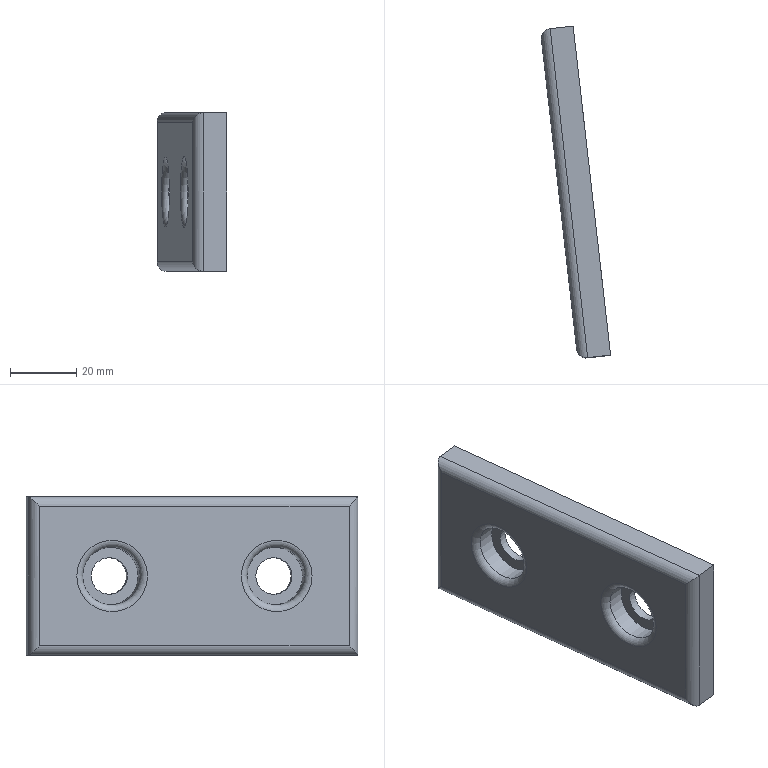Part | NX | features solid 2 | 1 solid | 18 faces | box 20.936 x 100.169 x 48 mm | volume 43256 mm3 | plane 8 | cylinder 8 | torus 2 | commonest cylinder face diameters 6 x4 11 x2 17.5 x2
STEP:
#1=CARTESIAN_POINT('',(3461.731,359.26,-59.));
#2=VERTEX_POINT('',#1);
#3=CARTESIAN_POINT('',(3462.354,353.796,-59.));
#4=DIRECTION('',(-0.9936,-0.1132,0.));
#5=DIRECTION('',(-0.1132,0.9936,0.));
#6=AXIS2_PLACEMENT_3D('',#3,#4,#5);
#7=CIRCLE('',#6,5.5);
#8=EDGE_CURVE('',#2,#2,#7,.T.);
#9=ORIENTED_EDGE('',*,*,#8,.T.);
#10=EDGE_LOOP('',(#9));
#11=FACE_BOUND('',#10,.T.);
#12=CARTESIAN_POINT('',(3467.392,309.582,-59.));
#13=VERTEX_POINT('',#12);
#14=CARTESIAN_POINT('',(3468.014,304.117,-59.));
#15=DIRECTION('',(-0.9936,-0.1132,0.));
#16=DIRECTION('',(-0.1132,0.9936,0.));
#17=AXIS2_PLACEMENT_3D('',#14,#15,#16);
#18=CIRCLE('',#17,5.5);
#19=EDGE_CURVE('',#13,#13,#18,.T.);
#20=ORIENTED_EDGE('',*,*,#19,.T.);
#21=EDGE_LOOP('',(#20));
#22=FACE_BOUND('',#21,.T.);
#23=CARTESIAN_POINT('',(3470.844,279.278,-35.));
#24=VERTEX_POINT('',#23);
#25=CARTESIAN_POINT('',(3470.844,279.278,-83.));
#26=VERTEX_POINT('',#25);
#27=CARTESIAN_POINT('',(3470.844,279.278,-59.));
#28=DIRECTION('',(0.,0.,-1.));
#29=VECTOR('',#28,1000.);
#30=LINE('',#27,#29);
#31=EDGE_CURVE('',#24,#26,#30,.T.);
#32=ORIENTED_EDGE('',*,*,#31,.T.);
#33=CARTESIAN_POINT('',(3459.524,378.635,-83.));
#34=VERTEX_POINT('',#33);
#35=CARTESIAN_POINT('',(3456.694,403.474,-83.));
#36=DIRECTION('',(0.1132,-0.9936,0.));
#37=VECTOR('',#36,1000.);
#38=LINE('',#35,#37);
#39=EDGE_CURVE('',#34,#26,#38,.T.);
#40=ORIENTED_EDGE('',*,*,#39,.F.);
#41=CARTESIAN_POINT('',(3459.524,378.635,-35.));
#42=VERTEX_POINT('',#41);
#43=CARTESIAN_POINT('',(3459.524,378.635,-59.));
#44=DIRECTION('',(0.,0.,1.));
#45=VECTOR('',#44,1000.);
#46=LINE('',#43,#45);
#47=EDGE_CURVE('',#34,#42,#46,.T.);
#48=ORIENTED_EDGE('',*,*,#47,.T.);
#49=CARTESIAN_POINT('',(3456.694,403.474,-35.));
#50=DIRECTION('',(0.1132,-0.9936,0.));
#51=VECTOR('',#50,1000.);
#52=LINE('',#49,#51);
#53=EDGE_CURVE('',#42,#24,#52,.T.);
#54=ORIENTED_EDGE('',*,*,#53,.T.);
#55=EDGE_LOOP('',(#32,#40,#48,#54));
#56=FACE_BOUND('',#55,.T.);
#57=CARTESIAN_POINT('',(3456.694,403.474,-59.));
#58=DIRECTION('',(0.9936,0.1132,0.));
#59=DIRECTION('',(0.1132,-0.9936,0.));
#60=AXIS2_PLACEMENT_3D('',#57,#58,#59);
#61=PLANE('',#60);
#62=ADVANCED_FACE('',(#11,#22,#56),#61,.T.);
#63=ORIENTED_EDGE('',*,*,#39,.T.);
#64=CARTESIAN_POINT('',(3463.889,278.485,-83.));
#65=VERTEX_POINT('',#64);
#66=CARTESIAN_POINT('',(3465.876,278.712,-83.));
#67=DIRECTION('',(-0.9936,-0.1132,0.));
#68=VECTOR('',#67,1000.);
#69=LINE('',#66,#68);
#70=EDGE_CURVE('',#26,#65,#69,.T.);
#71=ORIENTED_EDGE('',*,*,#70,.T.);
#72=CARTESIAN_POINT('',(3452.569,377.842,-83.));
#73=VERTEX_POINT('',#72);
#74=CARTESIAN_POINT('',(3449.739,402.682,-83.));
#75=DIRECTION('',(-0.1132,0.9936,0.));
#76=VECTOR('',#75,1000.);
#77=LINE('',#74,#76);
#78=EDGE_CURVE('',#65,#73,#77,.T.);
#79=ORIENTED_EDGE('',*,*,#78,.T.);
#80=CARTESIAN_POINT('',(3454.556,378.069,-83.));
#81=DIRECTION('',(0.9936,0.1132,0.));
#82=VECTOR('',#81,1000.);
#83=LINE('',#80,#82);
#84=EDGE_CURVE('',#73,#34,#83,.T.);
#85=ORIENTED_EDGE('',*,*,#84,.T.);
#86=EDGE_LOOP('',(#63,#71,#79,#85));
#87=FACE_BOUND('',#86,.T.);
#88=CARTESIAN_POINT('',(3451.726,402.908,-83.));
#89=DIRECTION('',(0.,0.,-1.));
#90=DIRECTION('',(-0.1132,0.9936,0.));
#91=AXIS2_PLACEMENT_3D('',#88,#89,#90);
#92=PLANE('',#91);
#93=ADVANCED_FACE('',(#87),#92,.T.);
#94=ORIENTED_EDGE('',*,*,#31,.F.);
#95=CARTESIAN_POINT('',(3463.889,278.485,-35.));
#96=VERTEX_POINT('',#95);
#97=CARTESIAN_POINT('',(3465.876,278.712,-35.));
#98=DIRECTION('',(0.9936,0.1132,0.));
#99=VECTOR('',#98,1000.);
#100=LINE('',#97,#99);
#101=EDGE_CURVE('',#96,#24,#100,.T.);
#102=ORIENTED_EDGE('',*,*,#101,.F.);
#103=CARTESIAN_POINT('',(3463.889,278.485,-59.));
#104=DIRECTION('',(0.,0.,-1.));
#105=VECTOR('',#104,1000.);
#106=LINE('',#103,#105);
#107=EDGE_CURVE('',#96,#65,#106,.T.);
#108=ORIENTED_EDGE('',*,*,#107,.T.);
#109=ORIENTED_EDGE('',*,*,#70,.F.);
#110=EDGE_LOOP('',(#94,#102,#108,#109));
#111=FACE_BOUND('',#110,.T.);
#112=CARTESIAN_POINT('',(3465.876,278.712,-59.));
#113=DIRECTION('',(0.1132,-0.9936,0.));
#114=DIRECTION('',(0.,0.,-1.));
#115=AXIS2_PLACEMENT_3D('',#112,#113,#114);
#116=PLANE('',#115);
#117=ADVANCED_FACE('',(#111),#116,.T.);
#118=CARTESIAN_POINT('',(3456.862,313.666,-59.));
#119=VERTEX_POINT('',#118);
#120=CARTESIAN_POINT('',(3458.078,302.985,-59.));
#121=DIRECTION('',(0.9936,0.1132,0.));
#122=DIRECTION('',(-0.1132,0.9936,0.));
#123=AXIS2_PLACEMENT_3D('',#120,#121,#122);
#124=CIRCLE('',#123,10.75);
#125=EDGE_CURVE('',#119,#119,#124,.T.);
#126=ORIENTED_EDGE('',*,*,#125,.T.);
#127=EDGE_LOOP('',(#126));
#128=FACE_BOUND('',#127,.T.);
#129=CARTESIAN_POINT('',(3451.201,363.344,-59.));
#130=VERTEX_POINT('',#129);
#131=CARTESIAN_POINT('',(3452.418,352.664,-59.));
#132=DIRECTION('',(0.9936,0.1132,0.));
#133=DIRECTION('',(-0.1132,0.9936,0.));
#134=AXIS2_PLACEMENT_3D('',#131,#132,#133);
#135=CIRCLE('',#134,10.75);
#136=EDGE_CURVE('',#130,#130,#135,.T.);
#137=ORIENTED_EDGE('',*,*,#136,.T.);
#138=EDGE_LOOP('',(#137));
#139=FACE_BOUND('',#138,.T.);
#140=CARTESIAN_POINT('',(3460.569,281.126,-38.));
#141=VERTEX_POINT('',#140);
#142=CARTESIAN_POINT('',(3449.928,374.522,-38.));
#143=VERTEX_POINT('',#142);
#144=CARTESIAN_POINT('',(3446.758,402.342,-38.));
#145=DIRECTION('',(-0.1132,0.9936,0.));
#146=VECTOR('',#145,1000.);
#147=LINE('',#144,#146);
#148=EDGE_CURVE('',#141,#143,#147,.T.);
#149=ORIENTED_EDGE('',*,*,#148,.T.);
#150=CARTESIAN_POINT('',(3449.928,374.522,-80.));
#151=VERTEX_POINT('',#150);
#152=CARTESIAN_POINT('',(3449.928,374.522,-59.));
#153=DIRECTION('',(0.,0.,-1.));
#154=VECTOR('',#153,1000.);
#155=LINE('',#152,#154);
#156=EDGE_CURVE('',#143,#151,#155,.T.);
#157=ORIENTED_EDGE('',*,*,#156,.T.);
#158=CARTESIAN_POINT('',(3460.569,281.126,-80.));
#159=VERTEX_POINT('',#158);
#160=CARTESIAN_POINT('',(3446.758,402.342,-80.));
#161=DIRECTION('',(0.1132,-0.9936,0.));
#162=VECTOR('',#161,1000.);
#163=LINE('',#160,#162);
#164=EDGE_CURVE('',#151,#159,#163,.T.);
#165=ORIENTED_EDGE('',*,*,#164,.T.);
#166=CARTESIAN_POINT('',(3460.569,281.126,-59.));
#167=DIRECTION('',(0.,0.,1.));
#168=VECTOR('',#167,1000.);
#169=LINE('',#166,#168);
#170=EDGE_CURVE('',#159,#141,#169,.T.);
#171=ORIENTED_EDGE('',*,*,#170,.T.);
#172=EDGE_LOOP('',(#149,#157,#165,#171));
#173=FACE_BOUND('',#172,.T.);
#174=CARTESIAN_POINT('',(3446.758,402.342,-59.));
#175=DIRECTION('',(-0.9936,-0.1132,0.));
#176=DIRECTION('',(-0.1132,0.9936,0.));
#177=AXIS2_PLACEMENT_3D('',#174,#175,#176);
#178=PLANE('',#177);
#179=ADVANCED_FACE('',(#128,#139,#173),#178,.T.);
#180=ORIENTED_EDGE('',*,*,#53,.F.);
#181=CARTESIAN_POINT('',(3452.569,377.842,-35.));
#182=VERTEX_POINT('',#181);
#183=CARTESIAN_POINT('',(3454.556,378.069,-35.));
#184=DIRECTION('',(-0.9936,-0.1132,0.));
#185=VECTOR('',#184,1000.);
#186=LINE('',#183,#185);
#187=EDGE_CURVE('',#42,#182,#186,.T.);
#188=ORIENTED_EDGE('',*,*,#187,.T.);
#189=CARTESIAN_POINT('',(3449.739,402.682,-35.));
#190=DIRECTION('',(0.1132,-0.9936,0.));
#191=VECTOR('',#190,1000.);
#192=LINE('',#189,#191);
#193=EDGE_CURVE('',#182,#96,#192,.T.);
#194=ORIENTED_EDGE('',*,*,#193,.T.);
#195=ORIENTED_EDGE('',*,*,#101,.T.);
#196=EDGE_LOOP('',(#180,#188,#194,#195));
#197=FACE_BOUND('',#196,.T.);
#198=CARTESIAN_POINT('',(3451.726,402.908,-35.));
#199=DIRECTION('',(0.,0.,1.));
#200=DIRECTION('',(0.1132,-0.9936,0.));
#201=AXIS2_PLACEMENT_3D('',#198,#199,#200);
#202=PLANE('',#201);
#203=ADVANCED_FACE('',(#197),#202,.T.);
#204=ORIENTED_EDGE('',*,*,#47,.F.);
#205=ORIENTED_EDGE('',*,*,#84,.F.);
#206=CARTESIAN_POINT('',(3452.569,377.842,-59.));
#207=DIRECTION('',(0.,0.,1.));
#208=VECTOR('',#207,1000.);
#209=LINE('',#206,#208);
#210=EDGE_CURVE('',#73,#182,#209,.T.);
#211=ORIENTED_EDGE('',*,*,#210,.T.);
#212=ORIENTED_EDGE('',*,*,#187,.F.);
#213=EDGE_LOOP('',(#204,#205,#211,#212));
#214=FACE_BOUND('',#213,.T.);
#215=CARTESIAN_POINT('',(3454.556,378.069,-59.));
#216=DIRECTION('',(-0.1132,0.9936,0.));
#217=DIRECTION('',(0.,0.,1.));
#218=AXIS2_PLACEMENT_3D('',#215,#216,#217);
#219=PLANE('',#218);
#220=ADVANCED_FACE('',(#214),#219,.T.);
#221=CARTESIAN_POINT('',(3463.55,281.466,-80.));
#222=DIRECTION('',(-0.08005,0.7026,-0.7071));
#223=DIRECTION('',(-0.08005,0.7026,0.7071));
#224=AXIS2_PLACEMENT_3D('',#221,#222,#223);
#225=ELLIPSE('',#224,4.243,3.);
#226=EDGE_CURVE('',#65,#159,#225,.T.);
#227=ORIENTED_EDGE('',*,*,#226,.F.);
#228=ORIENTED_EDGE('',*,*,#107,.F.);
#229=CARTESIAN_POINT('',(3463.55,281.466,-38.));
#230=DIRECTION('',(-0.08005,0.7026,0.7071));
#231=DIRECTION('',(0.08005,-0.7026,0.7071));
#232=AXIS2_PLACEMENT_3D('',#229,#230,#231);
#233=ELLIPSE('',#232,4.243,3.);
#234=EDGE_CURVE('',#141,#96,#233,.T.);
#235=ORIENTED_EDGE('',*,*,#234,.F.);
#236=ORIENTED_EDGE('',*,*,#170,.F.);
#237=EDGE_LOOP('',(#227,#228,#235,#236));
#238=FACE_BOUND('',#237,.T.);
#239=CARTESIAN_POINT('',(3463.55,281.466,-59.));
#240=DIRECTION('',(0.,0.,1.));
#241=DIRECTION('',(0.1132,-0.9936,0.));
#242=AXIS2_PLACEMENT_3D('',#239,#240,#241);
#243=CYLINDRICAL_SURFACE('',#242,3.);
#244=ADVANCED_FACE('',(#238),#243,.T.);
#245=ORIENTED_EDGE('',*,*,#234,.T.);
#246=ORIENTED_EDGE('',*,*,#193,.F.);
#247=CARTESIAN_POINT('',(3452.909,374.862,-38.));
#248=DIRECTION('',(-0.08005,0.7026,-0.7071));
#249=DIRECTION('',(0.08005,-0.7026,-0.7071));
#250=AXIS2_PLACEMENT_3D('',#247,#248,#249);
#251=ELLIPSE('',#250,4.243,3.);
#252=EDGE_CURVE('',#143,#182,#251,.T.);
#253=ORIENTED_EDGE('',*,*,#252,.F.);
#254=ORIENTED_EDGE('',*,*,#148,.F.);
#255=EDGE_LOOP('',(#245,#246,#253,#254));
#256=FACE_BOUND('',#255,.T.);
#257=CARTESIAN_POINT('',(3449.739,402.682,-38.));
#258=DIRECTION('',(0.1132,-0.9936,0.));
#259=DIRECTION('',(0.,0.,-1.));
#260=AXIS2_PLACEMENT_3D('',#257,#258,#259);
#261=CYLINDRICAL_SURFACE('',#260,3.);
#262=ADVANCED_FACE('',(#256),#261,.T.);
#263=ORIENTED_EDGE('',*,*,#226,.T.);
#264=ORIENTED_EDGE('',*,*,#164,.F.);
#265=CARTESIAN_POINT('',(3452.909,374.862,-80.));
#266=DIRECTION('',(-0.08005,0.7026,0.7071));
#267=DIRECTION('',(0.08005,-0.7026,0.7071));
#268=AXIS2_PLACEMENT_3D('',#265,#266,#267);
#269=ELLIPSE('',#268,4.243,3.);
#270=EDGE_CURVE('',#73,#151,#269,.T.);
#271=ORIENTED_EDGE('',*,*,#270,.F.);
#272=ORIENTED_EDGE('',*,*,#78,.F.);
#273=EDGE_LOOP('',(#263,#264,#271,#272));
#274=FACE_BOUND('',#273,.T.);
#275=CARTESIAN_POINT('',(3449.739,402.682,-80.));
#276=DIRECTION('',(0.1132,-0.9936,0.));
#277=DIRECTION('',(0.,0.,-1.));
#278=AXIS2_PLACEMENT_3D('',#275,#276,#277);
#279=CYLINDRICAL_SURFACE('',#278,3.);
#280=ADVANCED_FACE('',(#274),#279,.T.);
#281=ORIENTED_EDGE('',*,*,#252,.T.);
#282=ORIENTED_EDGE('',*,*,#210,.F.);
#283=ORIENTED_EDGE('',*,*,#270,.T.);
#284=ORIENTED_EDGE('',*,*,#156,.F.);
#285=EDGE_LOOP('',(#281,#282,#283,#284));
#286=FACE_BOUND('',#285,.T.);
#287=CARTESIAN_POINT('',(3452.909,374.862,-59.));
#288=DIRECTION('',(0.,0.,-1.));
#289=DIRECTION('',(-0.1132,0.9936,0.));
#290=AXIS2_PLACEMENT_3D('',#287,#288,#289);
#291=CYLINDRICAL_SURFACE('',#290,3.);
#292=ADVANCED_FACE('',(#286),#291,.T.);
#293=CARTESIAN_POINT('',(3460.493,348.048,-59.));
#294=VERTEX_POINT('',#293);
#295=CARTESIAN_POINT('',(3459.87,353.513,-59.));
#296=DIRECTION('',(0.9936,0.1132,0.));
#297=DIRECTION('',(0.1132,-0.9936,0.));
#298=AXIS2_PLACEMENT_3D('',#295,#296,#297);
#299=CIRCLE('',#298,5.5);
#300=EDGE_CURVE('',#294,#294,#299,.T.);
#301=ORIENTED_EDGE('',*,*,#300,.T.);
#302=EDGE_LOOP('',(#301));
#303=FACE_BOUND('',#302,.T.);
#304=CARTESIAN_POINT('',(3458.88,362.206,-59.));
#305=VERTEX_POINT('',#304);
#306=CARTESIAN_POINT('',(3459.87,353.513,-59.));
#307=DIRECTION('',(0.9936,0.1132,0.));
#308=DIRECTION('',(-0.1132,0.9936,0.));
#309=AXIS2_PLACEMENT_3D('',#306,#307,#308);
#310=CIRCLE('',#309,8.75);
#311=EDGE_CURVE('',#305,#305,#310,.T.);
#312=ORIENTED_EDGE('',*,*,#311,.F.);
#313=EDGE_LOOP('',(#312));
#314=FACE_BOUND('',#313,.T.);
#315=CARTESIAN_POINT('',(3459.87,353.513,-59.));
#316=DIRECTION('',(0.9936,0.1132,0.));
#317=DIRECTION('',(0.1132,-0.9936,0.));
#318=AXIS2_PLACEMENT_3D('',#315,#316,#317);
#319=PLANE('',#318);
#320=ADVANCED_FACE('',(#303,#314),#319,.F.);
#321=CARTESIAN_POINT('',(3453.415,361.584,-59.));
#322=VERTEX_POINT('',#321);
#323=CARTESIAN_POINT('',(3454.405,352.89,-59.));
#324=DIRECTION('',(-0.9936,-0.1132,0.));
#325=DIRECTION('',(-0.1132,0.9936,0.));
#326=AXIS2_PLACEMENT_3D('',#323,#324,#325);
#327=CIRCLE('',#326,8.75);
#328=EDGE_CURVE('',#322,#322,#327,.T.);
#329=ORIENTED_EDGE('',*,*,#328,.T.);
#330=EDGE_LOOP('',(#329));
#331=FACE_BOUND('',#330,.T.);
#332=ORIENTED_EDGE('',*,*,#311,.T.);
#333=EDGE_LOOP('',(#332));
#334=FACE_BOUND('',#333,.T.);
#335=CARTESIAN_POINT('',(3452.418,352.664,-59.));
#336=DIRECTION('',(0.9936,0.1132,0.));
#337=DIRECTION('',(0.1132,-0.9936,0.));
#338=AXIS2_PLACEMENT_3D('',#335,#336,#337);
#339=CYLINDRICAL_SURFACE('',#338,8.75);
#340=ADVANCED_FACE('',(#331,#334),#339,.F.);
#341=ORIENTED_EDGE('',*,*,#8,.F.);
#342=EDGE_LOOP('',(#341));
#343=FACE_BOUND('',#342,.T.);
#344=ORIENTED_EDGE('',*,*,#300,.F.);
#345=EDGE_LOOP('',(#344));
#346=FACE_BOUND('',#345,.T.);
#347=CARTESIAN_POINT('',(3452.418,352.664,-59.));
#348=DIRECTION('',(0.9936,0.1132,0.));
#349=DIRECTION('',(0.1132,-0.9936,0.));
#350=AXIS2_PLACEMENT_3D('',#347,#348,#349);
#351=CYLINDRICAL_SURFACE('',#350,5.5);
#352=ADVANCED_FACE('',(#343,#346),#351,.F.);
#353=CARTESIAN_POINT('',(3466.153,298.369,-59.));
#354=VERTEX_POINT('',#353);
#355=CARTESIAN_POINT('',(3465.53,303.834,-59.));
#356=DIRECTION('',(0.9936,0.1132,0.));
#357=DIRECTION('',(0.1132,-0.9936,0.));
#358=AXIS2_PLACEMENT_3D('',#355,#356,#357);
#359=CIRCLE('',#358,5.5);
#360=EDGE_CURVE('',#354,#354,#359,.T.);
#361=ORIENTED_EDGE('',*,*,#360,.T.);
#362=EDGE_LOOP('',(#361));
#363=FACE_BOUND('',#362,.T.);
#364=CARTESIAN_POINT('',(3464.54,312.528,-59.));
#365=VERTEX_POINT('',#364);
#366=CARTESIAN_POINT('',(3465.53,303.834,-59.));
#367=DIRECTION('',(0.9936,0.1132,0.));
#368=DIRECTION('',(-0.1132,0.9936,0.));
#369=AXIS2_PLACEMENT_3D('',#366,#367,#368);
#370=CIRCLE('',#369,8.75);
#371=EDGE_CURVE('',#365,#365,#370,.T.);
#372=ORIENTED_EDGE('',*,*,#371,.F.);
#373=EDGE_LOOP('',(#372));
#374=FACE_BOUND('',#373,.T.);
#375=CARTESIAN_POINT('',(3465.53,303.834,-59.));
#376=DIRECTION('',(0.9936,0.1132,0.));
#377=DIRECTION('',(0.1132,-0.9936,0.));
#378=AXIS2_PLACEMENT_3D('',#375,#376,#377);
#379=PLANE('',#378);
#380=ADVANCED_FACE('',(#363,#374),#379,.F.);
#381=CARTESIAN_POINT('',(3459.075,311.905,-59.));
#382=VERTEX_POINT('',#381);
#383=CARTESIAN_POINT('',(3460.066,303.211,-59.));
#384=DIRECTION('',(-0.9936,-0.1132,0.));
#385=DIRECTION('',(-0.1132,0.9936,0.));
#386=AXIS2_PLACEMENT_3D('',#383,#384,#385);
#387=CIRCLE('',#386,8.75);
#388=EDGE_CURVE('',#382,#382,#387,.T.);
#389=ORIENTED_EDGE('',*,*,#388,.T.);
#390=EDGE_LOOP('',(#389));
#391=FACE_BOUND('',#390,.T.);
#392=ORIENTED_EDGE('',*,*,#371,.T.);
#393=EDGE_LOOP('',(#392));
#394=FACE_BOUND('',#393,.T.);
#395=CARTESIAN_POINT('',(3458.078,302.985,-59.));
#396=DIRECTION('',(0.9936,0.1132,0.));
#397=DIRECTION('',(0.1132,-0.9936,0.));
#398=AXIS2_PLACEMENT_3D('',#395,#396,#397);
#399=CYLINDRICAL_SURFACE('',#398,8.75);
#400=ADVANCED_FACE('',(#391,#394),#399,.F.);
#401=ORIENTED_EDGE('',*,*,#19,.F.);
#402=EDGE_LOOP('',(#401));
#403=FACE_BOUND('',#402,.T.);
#404=ORIENTED_EDGE('',*,*,#360,.F.);
#405=EDGE_LOOP('',(#404));
#406=FACE_BOUND('',#405,.T.);
#407=CARTESIAN_POINT('',(3458.078,302.985,-59.));
#408=DIRECTION('',(0.9936,0.1132,0.));
#409=DIRECTION('',(0.1132,-0.9936,0.));
#410=AXIS2_PLACEMENT_3D('',#407,#408,#409);
#411=CYLINDRICAL_SURFACE('',#410,5.5);
#412=ADVANCED_FACE('',(#403,#406),#411,.F.);
#413=ORIENTED_EDGE('',*,*,#328,.F.);
#414=EDGE_LOOP('',(#413));
#415=FACE_BOUND('',#414,.T.);
#416=ORIENTED_EDGE('',*,*,#136,.F.);
#417=EDGE_LOOP('',(#416));
#418=FACE_BOUND('',#417,.T.);
#419=CARTESIAN_POINT('',(3454.405,352.89,-59.));
#420=DIRECTION('',(-0.9936,-0.1132,0.));
#421=DIRECTION('',(-0.1132,0.9936,0.));
#422=AXIS2_PLACEMENT_3D('',#419,#420,#421);
#423=TOROIDAL_SURFACE('',#422,10.75,2.);
#424=ADVANCED_FACE('',(#415,#418),#423,.T.);
#425=ORIENTED_EDGE('',*,*,#388,.F.);
#426=EDGE_LOOP('',(#425));
#427=FACE_BOUND('',#426,.T.);
#428=ORIENTED_EDGE('',*,*,#125,.F.);
#429=EDGE_LOOP('',(#428));
#430=FACE_BOUND('',#429,.T.);
#431=CARTESIAN_POINT('',(3460.066,303.211,-59.));
#432=DIRECTION('',(-0.9936,-0.1132,0.));
#433=DIRECTION('',(-0.1132,0.9936,0.));
#434=AXIS2_PLACEMENT_3D('',#431,#432,#433);
#435=TOROIDAL_SURFACE('',#434,10.75,2.);
#436=ADVANCED_FACE('',(#427,#430),#435,.T.);
#437=CLOSED_SHELL('',(#62,#93,#117,#179,#203,#220,#244,#262,#280,#292,#320,#340,#352,#380,#400,#412,#424,#436));
#438=MANIFOLD_SOLID_BREP('',#437);
#439=(LENGTH_UNIT()NAMED_UNIT(*)SI_UNIT(.MILLI.,.METRE.));
#440=UNCERTAINTY_MEASURE_WITH_UNIT(LENGTH_MEASURE(0.00001),#439,'','');
#441=(NAMED_UNIT(*)PLANE_ANGLE_UNIT()SI_UNIT($,.RADIAN.));
#442=(NAMED_UNIT(*)SI_UNIT($,.STERADIAN.)SOLID_ANGLE_UNIT());
#443=(GEOMETRIC_REPRESENTATION_CONTEXT(3)GLOBAL_UNCERTAINTY_ASSIGNED_CONTEXT((#440))GLOBAL_UNIT_ASSIGNED_CONTEXT((#439,#441,#442))REPRESENTATION_CONTEXT('',''));
#444=ADVANCED_BREP_SHAPE_REPRESENTATION('',(#438),#443);